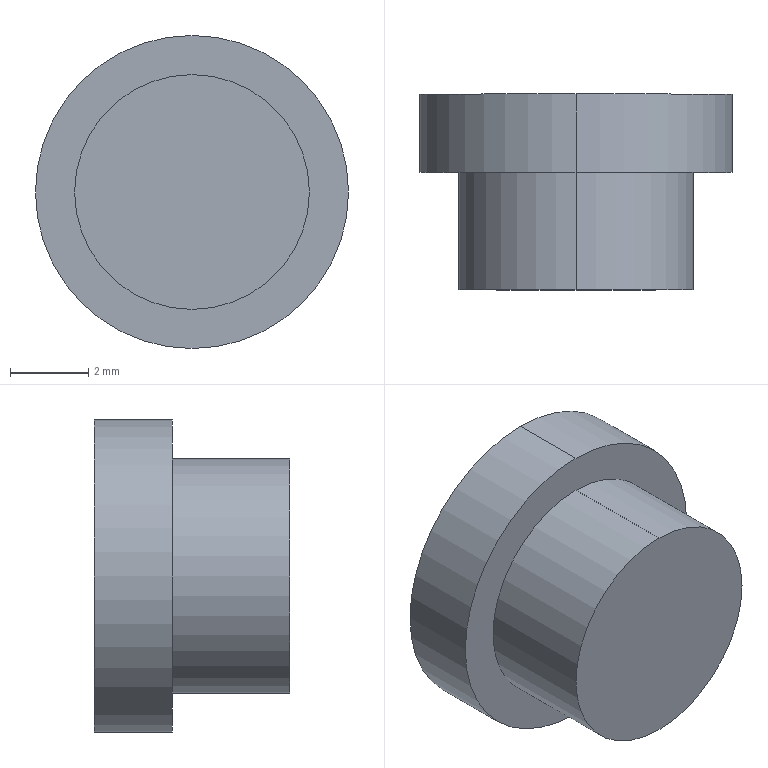Part | SolidWorks | features Revolution 1 | 1 solid | 7 faces | box 8 x 5 x 8 mm | volume 185.354 mm3 | cylinder 4 | plane 3 | commonest cylinder face diameters 6 x2 8 x2
STEP:
#1=CARTESIAN_POINT('',(0.,-2.,-3.));
#2=VERTEX_POINT('',#1);
#3=CARTESIAN_POINT('',(0.,-2.,3.));
#4=VERTEX_POINT('',#3);
#5=CARTESIAN_POINT('',(0.,-2.,0.));
#6=DIRECTION('',(0.,-1.,0.));
#7=DIRECTION('',(0.,0.,-1.));
#8=AXIS2_PLACEMENT_3D('',#5,#6,#7);
#9=CIRCLE('',#8,3.);
#10=EDGE_CURVE('',#2,#4,#9,.T.);
#11=ORIENTED_EDGE('',*,*,#10,.T.);
#12=CARTESIAN_POINT('',(0.,-5.,3.));
#13=VERTEX_POINT('',#12);
#14=CARTESIAN_POINT('',(0.,-5.,3.));
#15=DIRECTION('',(0.,-1.,0.));
#16=VECTOR('',#15,1000.);
#17=LINE('',#14,#16);
#18=EDGE_CURVE('',#4,#13,#17,.T.);
#19=ORIENTED_EDGE('',*,*,#18,.T.);
#20=CARTESIAN_POINT('',(0.,-5.,-3.));
#21=VERTEX_POINT('',#20);
#22=CARTESIAN_POINT('',(0.,-5.,0.));
#23=DIRECTION('',(0.,-1.,0.));
#24=DIRECTION('',(0.,0.,-1.));
#25=AXIS2_PLACEMENT_3D('',#22,#23,#24);
#26=CIRCLE('',#25,3.);
#27=EDGE_CURVE('',#21,#13,#26,.T.);
#28=ORIENTED_EDGE('',*,*,#27,.F.);
#29=CARTESIAN_POINT('',(0.,-5.,-3.));
#30=DIRECTION('',(0.,-1.,0.));
#31=VECTOR('',#30,1000.);
#32=LINE('',#29,#31);
#33=EDGE_CURVE('',#2,#21,#32,.T.);
#34=ORIENTED_EDGE('',*,*,#33,.F.);
#35=EDGE_LOOP('',(#11,#19,#28,#34));
#36=FACE_OUTER_BOUND('',#35,.T.);
#37=CARTESIAN_POINT('',(0.,-5.,0.));
#38=DIRECTION('',(0.,-1.,0.));
#39=DIRECTION('',(0.,0.,-1.));
#40=AXIS2_PLACEMENT_3D('',#37,#38,#39);
#41=CYLINDRICAL_SURFACE('',#40,3.);
#42=ADVANCED_FACE('',(#36),#41,.T.);
#43=CARTESIAN_POINT('',(0.,0.,-4.));
#44=VERTEX_POINT('',#43);
#45=CARTESIAN_POINT('',(0.,0.,4.));
#46=VERTEX_POINT('',#45);
#47=CARTESIAN_POINT('',(0.,0.,0.));
#48=DIRECTION('',(0.,-1.,0.));
#49=DIRECTION('',(0.,0.,-1.));
#50=AXIS2_PLACEMENT_3D('',#47,#48,#49);
#51=CIRCLE('',#50,4.);
#52=EDGE_CURVE('',#44,#46,#51,.T.);
#53=ORIENTED_EDGE('',*,*,#52,.T.);
#54=CARTESIAN_POINT('',(0.,-2.,4.));
#55=VERTEX_POINT('',#54);
#56=CARTESIAN_POINT('',(0.,-5.,4.));
#57=DIRECTION('',(0.,-1.,0.));
#58=VECTOR('',#57,1000.);
#59=LINE('',#56,#58);
#60=EDGE_CURVE('',#46,#55,#59,.T.);
#61=ORIENTED_EDGE('',*,*,#60,.T.);
#62=CARTESIAN_POINT('',(0.,-2.,-4.));
#63=VERTEX_POINT('',#62);
#64=CARTESIAN_POINT('',(0.,-2.,0.));
#65=DIRECTION('',(0.,-1.,0.));
#66=DIRECTION('',(0.,0.,-1.));
#67=AXIS2_PLACEMENT_3D('',#64,#65,#66);
#68=CIRCLE('',#67,4.);
#69=EDGE_CURVE('',#63,#55,#68,.T.);
#70=ORIENTED_EDGE('',*,*,#69,.F.);
#71=CARTESIAN_POINT('',(0.,-5.,-4.));
#72=DIRECTION('',(0.,-1.,0.));
#73=VECTOR('',#72,1000.);
#74=LINE('',#71,#73);
#75=EDGE_CURVE('',#44,#63,#74,.T.);
#76=ORIENTED_EDGE('',*,*,#75,.F.);
#77=EDGE_LOOP('',(#53,#61,#70,#76));
#78=FACE_OUTER_BOUND('',#77,.T.);
#79=CARTESIAN_POINT('',(0.,-5.,0.));
#80=DIRECTION('',(0.,-1.,0.));
#81=DIRECTION('',(0.,0.,-1.));
#82=AXIS2_PLACEMENT_3D('',#79,#80,#81);
#83=CYLINDRICAL_SURFACE('',#82,4.);
#84=ADVANCED_FACE('',(#78),#83,.T.);
#85=ORIENTED_EDGE('',*,*,#52,.F.);
#86=CARTESIAN_POINT('',(0.,0.,0.));
#87=DIRECTION('',(0.,-1.,0.));
#88=DIRECTION('',(0.,0.,-1.));
#89=AXIS2_PLACEMENT_3D('',#86,#87,#88);
#90=CIRCLE('',#89,4.);
#91=EDGE_CURVE('',#46,#44,#90,.T.);
#92=ORIENTED_EDGE('',*,*,#91,.F.);
#93=EDGE_LOOP('',(#85,#92));
#94=FACE_OUTER_BOUND('',#93,.T.);
#95=CARTESIAN_POINT('',(0.,0.,0.));
#96=DIRECTION('',(0.,1.,0.));
#97=DIRECTION('',(0.,0.,1.));
#98=AXIS2_PLACEMENT_3D('',#95,#96,#97);
#99=PLANE('',#98);
#100=ADVANCED_FACE('',(#94),#99,.T.);
#101=ORIENTED_EDGE('',*,*,#60,.F.);
#102=ORIENTED_EDGE('',*,*,#91,.T.);
#103=ORIENTED_EDGE('',*,*,#75,.T.);
#104=CARTESIAN_POINT('',(0.,-2.,0.));
#105=DIRECTION('',(0.,-1.,0.));
#106=DIRECTION('',(0.,0.,-1.));
#107=AXIS2_PLACEMENT_3D('',#104,#105,#106);
#108=CIRCLE('',#107,4.);
#109=EDGE_CURVE('',#55,#63,#108,.T.);
#110=ORIENTED_EDGE('',*,*,#109,.F.);
#111=EDGE_LOOP('',(#101,#102,#103,#110));
#112=FACE_OUTER_BOUND('',#111,.T.);
#113=CARTESIAN_POINT('',(0.,-5.,0.));
#114=DIRECTION('',(0.,-1.,0.));
#115=DIRECTION('',(0.,0.,-1.));
#116=AXIS2_PLACEMENT_3D('',#113,#114,#115);
#117=CYLINDRICAL_SURFACE('',#116,4.);
#118=ADVANCED_FACE('',(#112),#117,.T.);
#119=ORIENTED_EDGE('',*,*,#69,.T.);
#120=ORIENTED_EDGE('',*,*,#109,.T.);
#121=EDGE_LOOP('',(#119,#120));
#122=FACE_OUTER_BOUND('',#121,.T.);
#123=ORIENTED_EDGE('',*,*,#10,.F.);
#124=CARTESIAN_POINT('',(0.,-2.,0.));
#125=DIRECTION('',(0.,-1.,0.));
#126=DIRECTION('',(0.,0.,-1.));
#127=AXIS2_PLACEMENT_3D('',#124,#125,#126);
#128=CIRCLE('',#127,3.);
#129=EDGE_CURVE('',#4,#2,#128,.T.);
#130=ORIENTED_EDGE('',*,*,#129,.F.);
#131=EDGE_LOOP('',(#123,#130));
#132=FACE_BOUND('',#131,.T.);
#133=CARTESIAN_POINT('',(4.,-2.,0.));
#134=DIRECTION('',(0.,-1.,0.));
#135=DIRECTION('',(0.,0.,-1.));
#136=AXIS2_PLACEMENT_3D('',#133,#134,#135);
#137=PLANE('',#136);
#138=ADVANCED_FACE('',(#122,#132),#137,.T.);
#139=ORIENTED_EDGE('',*,*,#18,.F.);
#140=ORIENTED_EDGE('',*,*,#129,.T.);
#141=ORIENTED_EDGE('',*,*,#33,.T.);
#142=CARTESIAN_POINT('',(0.,-5.,0.));
#143=DIRECTION('',(0.,-1.,0.));
#144=DIRECTION('',(0.,0.,-1.));
#145=AXIS2_PLACEMENT_3D('',#142,#143,#144);
#146=CIRCLE('',#145,3.);
#147=EDGE_CURVE('',#13,#21,#146,.T.);
#148=ORIENTED_EDGE('',*,*,#147,.F.);
#149=EDGE_LOOP('',(#139,#140,#141,#148));
#150=FACE_OUTER_BOUND('',#149,.T.);
#151=CARTESIAN_POINT('',(0.,-5.,0.));
#152=DIRECTION('',(0.,-1.,0.));
#153=DIRECTION('',(0.,0.,-1.));
#154=AXIS2_PLACEMENT_3D('',#151,#152,#153);
#155=CYLINDRICAL_SURFACE('',#154,3.);
#156=ADVANCED_FACE('',(#150),#155,.T.);
#157=ORIENTED_EDGE('',*,*,#27,.T.);
#158=ORIENTED_EDGE('',*,*,#147,.T.);
#159=EDGE_LOOP('',(#157,#158));
#160=FACE_OUTER_BOUND('',#159,.T.);
#161=CARTESIAN_POINT('',(3.,-5.,0.));
#162=DIRECTION('',(0.,-1.,0.));
#163=DIRECTION('',(0.,0.,-1.));
#164=AXIS2_PLACEMENT_3D('',#161,#162,#163);
#165=PLANE('',#164);
#166=ADVANCED_FACE('',(#160),#165,.T.);
#167=CLOSED_SHELL('',(#42,#84,#100,#118,#138,#156,#166));
#168=MANIFOLD_SOLID_BREP('',#167);
#169=CARTESIAN_POINT('',(0.,0.,0.));
#170=DIRECTION('',(0.,0.,1.));
#171=DIRECTION('',(1.,0.,0.));
#172=AXIS2_PLACEMENT_3D('',#169,#170,#171);
#173=(LENGTH_UNIT()NAMED_UNIT(*)SI_UNIT(.MILLI.,.METRE.));
#174=UNCERTAINTY_MEASURE_WITH_UNIT(LENGTH_MEASURE(0.00001),#173,'','');
#175=(NAMED_UNIT(*)PLANE_ANGLE_UNIT()SI_UNIT($,.RADIAN.));
#176=(NAMED_UNIT(*)SI_UNIT($,.STERADIAN.)SOLID_ANGLE_UNIT());
#177=(GEOMETRIC_REPRESENTATION_CONTEXT(3)GLOBAL_UNCERTAINTY_ASSIGNED_CONTEXT((#174))GLOBAL_UNIT_ASSIGNED_CONTEXT((#173,#175,#176))REPRESENTATION_CONTEXT('',''));
#178=ADVANCED_BREP_SHAPE_REPRESENTATION('',(#168,#172),#177);